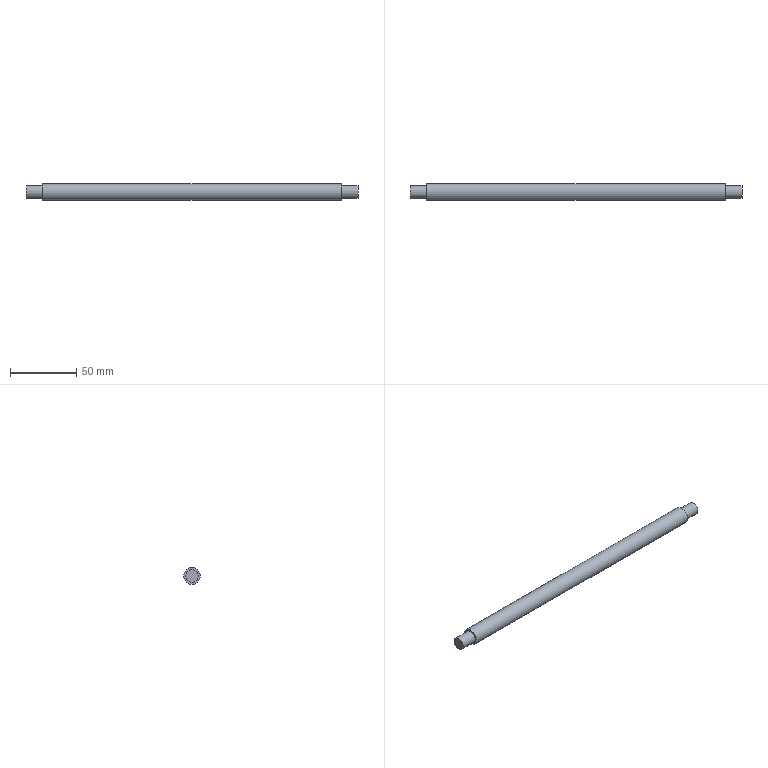Part | NX | features solid 2 | 1 solid | 7 faces | box 249.693 x 12.7 x 12.7 mm | volume 30223 mm3 | plane 4 | cylinder 3 | commonest cylinder face diameters 9.525 x2 12.7 x1
STEP:
#1=CARTESIAN_POINT('',(-124.847,0.,-4.763));
#2=VERTEX_POINT('',#1);
#3=CARTESIAN_POINT('',(-124.847,0.,0.));
#4=DIRECTION('',(1.,0.,0.));
#5=DIRECTION('',(0.,0.,-1.));
#6=AXIS2_PLACEMENT_3D('',#3,#4,#5);
#7=CIRCLE('',#6,4.763);
#8=EDGE_CURVE('',#2,#2,#7,.T.);
#9=ORIENTED_EDGE('',*,*,#8,.F.);
#10=EDGE_LOOP('',(#9));
#11=FACE_BOUND('',#10,.T.);
#12=CARTESIAN_POINT('',(-124.847,0.,0.));
#13=DIRECTION('',(1.,0.,0.));
#14=DIRECTION('',(0.,0.,-1.));
#15=AXIS2_PLACEMENT_3D('',#12,#13,#14);
#16=PLANE('',#15);
#17=ADVANCED_FACE('',(#11),#16,.F.);
#18=CARTESIAN_POINT('',(-112.147,0.,-4.763));
#19=VERTEX_POINT('',#18);
#20=CARTESIAN_POINT('',(-112.147,0.,0.));
#21=DIRECTION('',(1.,0.,0.));
#22=DIRECTION('',(0.,0.,-1.));
#23=AXIS2_PLACEMENT_3D('',#20,#21,#22);
#24=CIRCLE('',#23,4.763);
#25=EDGE_CURVE('',#19,#19,#24,.T.);
#26=ORIENTED_EDGE('',*,*,#25,.F.);
#27=EDGE_LOOP('',(#26));
#28=FACE_BOUND('',#27,.T.);
#29=ORIENTED_EDGE('',*,*,#8,.T.);
#30=EDGE_LOOP('',(#29));
#31=FACE_BOUND('',#30,.T.);
#32=CARTESIAN_POINT('',(-124.847,0.,0.));
#33=DIRECTION('',(1.,0.,0.));
#34=DIRECTION('',(0.,0.,-1.));
#35=AXIS2_PLACEMENT_3D('',#32,#33,#34);
#36=CYLINDRICAL_SURFACE('',#35,4.763);
#37=ADVANCED_FACE('',(#28,#31),#36,.T.);
#38=CARTESIAN_POINT('',(-112.147,0.,-6.35));
#39=VERTEX_POINT('',#38);
#40=CARTESIAN_POINT('',(-112.147,0.,0.));
#41=DIRECTION('',(1.,0.,0.));
#42=DIRECTION('',(0.,0.,-1.));
#43=AXIS2_PLACEMENT_3D('',#40,#41,#42);
#44=CIRCLE('',#43,6.35);
#45=EDGE_CURVE('',#39,#39,#44,.T.);
#46=ORIENTED_EDGE('',*,*,#45,.F.);
#47=EDGE_LOOP('',(#46));
#48=FACE_BOUND('',#47,.T.);
#49=ORIENTED_EDGE('',*,*,#25,.T.);
#50=EDGE_LOOP('',(#49));
#51=FACE_BOUND('',#50,.T.);
#52=CARTESIAN_POINT('',(-112.147,0.,-4.763));
#53=DIRECTION('',(1.,0.,0.));
#54=DIRECTION('',(0.,0.,-1.));
#55=AXIS2_PLACEMENT_3D('',#52,#53,#54);
#56=PLANE('',#55);
#57=ADVANCED_FACE('',(#48,#51),#56,.F.);
#58=CARTESIAN_POINT('',(112.147,0.,-6.35));
#59=VERTEX_POINT('',#58);
#60=CARTESIAN_POINT('',(112.147,0.,0.));
#61=DIRECTION('',(1.,0.,0.));
#62=DIRECTION('',(0.,0.,-1.));
#63=AXIS2_PLACEMENT_3D('',#60,#61,#62);
#64=CIRCLE('',#63,6.35);
#65=EDGE_CURVE('',#59,#59,#64,.T.);
#66=ORIENTED_EDGE('',*,*,#65,.F.);
#67=EDGE_LOOP('',(#66));
#68=FACE_BOUND('',#67,.T.);
#69=ORIENTED_EDGE('',*,*,#45,.T.);
#70=EDGE_LOOP('',(#69));
#71=FACE_BOUND('',#70,.T.);
#72=CARTESIAN_POINT('',(-124.847,0.,0.));
#73=DIRECTION('',(1.,0.,0.));
#74=DIRECTION('',(0.,0.,-1.));
#75=AXIS2_PLACEMENT_3D('',#72,#73,#74);
#76=CYLINDRICAL_SURFACE('',#75,6.35);
#77=ADVANCED_FACE('',(#68,#71),#76,.T.);
#78=CARTESIAN_POINT('',(112.147,0.,-4.763));
#79=VERTEX_POINT('',#78);
#80=CARTESIAN_POINT('',(112.147,0.,0.));
#81=DIRECTION('',(1.,0.,0.));
#82=DIRECTION('',(0.,0.,-1.));
#83=AXIS2_PLACEMENT_3D('',#80,#81,#82);
#84=CIRCLE('',#83,4.763);
#85=EDGE_CURVE('',#79,#79,#84,.T.);
#86=ORIENTED_EDGE('',*,*,#85,.F.);
#87=EDGE_LOOP('',(#86));
#88=FACE_BOUND('',#87,.T.);
#89=ORIENTED_EDGE('',*,*,#65,.T.);
#90=EDGE_LOOP('',(#89));
#91=FACE_BOUND('',#90,.T.);
#92=CARTESIAN_POINT('',(112.147,0.,-6.35));
#93=DIRECTION('',(-1.,0.,0.));
#94=DIRECTION('',(0.,0.,1.));
#95=AXIS2_PLACEMENT_3D('',#92,#93,#94);
#96=PLANE('',#95);
#97=ADVANCED_FACE('',(#88,#91),#96,.F.);
#98=CARTESIAN_POINT('',(124.847,0.,-4.763));
#99=VERTEX_POINT('',#98);
#100=CARTESIAN_POINT('',(124.847,0.,0.));
#101=DIRECTION('',(1.,0.,0.));
#102=DIRECTION('',(0.,0.,-1.));
#103=AXIS2_PLACEMENT_3D('',#100,#101,#102);
#104=CIRCLE('',#103,4.763);
#105=EDGE_CURVE('',#99,#99,#104,.T.);
#106=ORIENTED_EDGE('',*,*,#105,.F.);
#107=EDGE_LOOP('',(#106));
#108=FACE_BOUND('',#107,.T.);
#109=ORIENTED_EDGE('',*,*,#85,.T.);
#110=EDGE_LOOP('',(#109));
#111=FACE_BOUND('',#110,.T.);
#112=CARTESIAN_POINT('',(-124.847,0.,0.));
#113=DIRECTION('',(1.,0.,0.));
#114=DIRECTION('',(0.,0.,-1.));
#115=AXIS2_PLACEMENT_3D('',#112,#113,#114);
#116=CYLINDRICAL_SURFACE('',#115,4.763);
#117=ADVANCED_FACE('',(#108,#111),#116,.T.);
#118=ORIENTED_EDGE('',*,*,#105,.T.);
#119=EDGE_LOOP('',(#118));
#120=FACE_BOUND('',#119,.T.);
#121=CARTESIAN_POINT('',(124.847,0.,-4.763));
#122=DIRECTION('',(-1.,0.,0.));
#123=DIRECTION('',(0.,0.,1.));
#124=AXIS2_PLACEMENT_3D('',#121,#122,#123);
#125=PLANE('',#124);
#126=ADVANCED_FACE('',(#120),#125,.F.);
#127=CLOSED_SHELL('',(#17,#37,#57,#77,#97,#117,#126));
#128=MANIFOLD_SOLID_BREP('',#127);
#129=(LENGTH_UNIT()NAMED_UNIT(*)SI_UNIT(.MILLI.,.METRE.));
#130=UNCERTAINTY_MEASURE_WITH_UNIT(LENGTH_MEASURE(0.00001),#129,'','');
#131=(NAMED_UNIT(*)PLANE_ANGLE_UNIT()SI_UNIT($,.RADIAN.));
#132=(NAMED_UNIT(*)SI_UNIT($,.STERADIAN.)SOLID_ANGLE_UNIT());
#133=(GEOMETRIC_REPRESENTATION_CONTEXT(3)GLOBAL_UNCERTAINTY_ASSIGNED_CONTEXT((#130))GLOBAL_UNIT_ASSIGNED_CONTEXT((#129,#131,#132))REPRESENTATION_CONTEXT('',''));
#134=ADVANCED_BREP_SHAPE_REPRESENTATION('',(#128),#133);